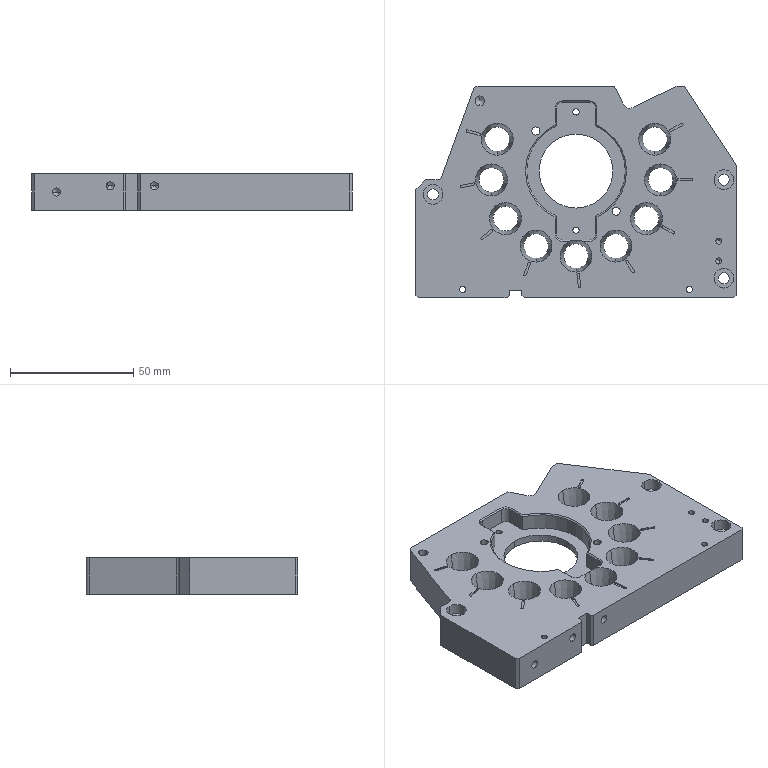NC program | NX | posted with a generic post | part box 130 x 86 x 15 mm
Lines 106 to 1053 of 51277:
(ZLEVEL_PROFILE , TOOL : D10)
N180 T04 M6
N182 G54
N184 G17 G0 G90 X48.294 Y-20.755 B0. C0. S3500 M3
N186 G43 Z30. H4
N188 Z-0.217
N190 G94 G1 X47.012 Y-19.892 F1000.
N192 G3 X46.014 Y-19.823 R1.
N194 G1 X45.265 Y-20.189 F2200.
N196 X39.925 Y-22.793
N198 X39.818 Y-22.842
N200 X47.584 Y-38.764
N202 G2 X48.1 Y-41. R5.1
N204 G1 Y-43.46
N206 G2 X45.347 Y-48.56 R6.1
N208 G1 X14.298 Y-68.936
N210 G2 X10.402 Y-70.1 R7.1
N212 G3 X9.536 Y-70.6 R1.
N214 G1 X8.67 Y-72.1
N216 G0 Z-0.435
N218 G1 X9.536 Y-70.6 F1000.
N220 G2 X10.402 Y-70.1 R1.
N222 G3 X14.298 Y-68.936 R7.1 F2200.
N224 G1 X45.347 Y-48.56
N226 G3 X48.1 Y-43.46 R6.1
N228 G1 Y-41.
N230 G3 X47.584 Y-38.764 R5.1
N232 G1 X39.818 Y-22.842
N234 X39.925 Y-22.793
N236 X45.265 Y-20.189
N238 X46.014 Y-19.823
N240 G2 X47.012 Y-19.892 R1.
N242 G1 X48.294 Y-20.755
N244 G0 Z-0.652
N246 G1 X47.012 Y-19.892 F1000.
N248 G3 X46.014 Y-19.823 R1.
N250 G1 X45.265 Y-20.189 F2200.
N252 X39.925 Y-22.793
N254 X39.818 Y-22.842
N256 X47.584 Y-38.764
N258 G2 X48.1 Y-41. R5.1
N260 G1 Y-43.46
N262 G2 X45.347 Y-48.56 R6.1
N264 G1 X14.298 Y-68.936
N266 G2 X10.402 Y-70.1 R7.1
N268 G3 X9.536 Y-70.6 R1.
N270 G1 X8.67 Y-72.1
N272 G0 Z-0.87
N274 G1 X9.536 Y-70.6 F1000.
N276 G2 X10.402 Y-70.1 R1.
N278 G3 X14.298 Y-68.936 R7.1 F2200.
N280 G1 X45.347 Y-48.56
N282 G3 X48.1 Y-43.46 R6.1
N284 G1 Y-41.
N286 G3 X47.584 Y-38.764 R5.1
N288 G1 X39.818 Y-22.842
N290 X39.925 Y-22.793
N292 X45.265 Y-20.189
N294 X46.014 Y-19.823
N296 G2 X47.012 Y-19.892 R1.
N298 G1 X48.294 Y-20.755
N300 G0 Z-1.087
N302 G1 X47.012 Y-19.892 F1000.
N304 G3 X46.014 Y-19.823 R1.
N306 G1 X45.265 Y-20.189 F2200.
N308 X39.925 Y-22.793
N310 X39.818 Y-22.842
N312 X47.584 Y-38.764
N314 G2 X48.1 Y-41. R5.1
N316 G1 Y-43.46
N318 G2 X45.347 Y-48.56 R6.1
N320 G1 X14.298 Y-68.936
N322 G2 X10.402 Y-70.1 R7.1
N324 G3 X9.536 Y-70.6 R1.
N326 G1 X8.67 Y-72.1
N328 G0 Z-1.304
N330 G1 X9.536 Y-70.6 F1000.
N332 G2 X10.402 Y-70.1 R1.
N334 G3 X14.298 Y-68.936 R7.1 F2200.
N336 G1 X45.347 Y-48.56
N338 G3 X48.1 Y-43.46 R6.1
N340 G1 Y-41.
N342 G3 X47.584 Y-38.764 R5.1
N344 G1 X39.818 Y-22.842
N346 X39.925 Y-22.793
N348 X45.265 Y-20.189
N350 X46.014 Y-19.823
N352 G2 X47.012 Y-19.892 R1.
N354 G1 X48.294 Y-20.755
N356 G0 Z-1.522
N358 G1 X47.012 Y-19.892 F1000.
N360 G3 X46.014 Y-19.823 R1.
N362 G1 X45.265 Y-20.189 F2200.
N364 X39.925 Y-22.793
N366 X39.818 Y-22.842
N368 X47.584 Y-38.764
N370 G2 X48.1 Y-41. R5.1
N372 G1 Y-43.46
N374 G2 X45.347 Y-48.56 R6.1
N376 G1 X14.298 Y-68.936
N378 G2 X10.402 Y-70.1 R7.1
N380 G3 X9.536 Y-70.6 R1.
N382 G1 X8.67 Y-72.1
N384 G0 Z-1.739
N386 G1 X9.536 Y-70.6 F1000.
N388 G2 X10.402 Y-70.1 R1.
N390 G3 X14.298 Y-68.936 R7.1 F2200.
N392 G1 X45.347 Y-48.56
N394 G3 X48.1 Y-43.46 R6.1
N396 G1 Y-41.
N398 G3 X47.584 Y-38.764 R5.1
N400 G1 X39.818 Y-22.842
N402 X39.925 Y-22.793
N404 X45.265 Y-20.189
N406 X46.014 Y-19.823
N408 G2 X47.012 Y-19.892 R1.
N410 G1 X48.294 Y-20.756
N412 G0 Z-1.957
N414 G1 X47.012 Y-19.892 F1000.
N416 G3 X46.014 Y-19.823 R1.
N418 G1 X45.265 Y-20.189 F2200.
N420 X39.925 Y-22.793
N422 X39.818 Y-22.842
N424 X47.584 Y-38.764
N426 G2 X48.1 Y-41. R5.1
N428 G1 Y-43.46
N430 G2 X45.347 Y-48.56 R6.1
N432 G1 X14.298 Y-68.936
N434 G2 X10.402 Y-70.1 R7.1
N436 G3 X9.536 Y-70.6 R1.
N438 G1 X8.67 Y-72.1
N440 G0 Z-2.174
N442 G1 X9.536 Y-70.6 F1000.
N444 G2 X10.402 Y-70.1 R1.
N446 G3 X14.298 Y-68.936 R7.1 F2200.
N448 G1 X45.347 Y-48.56
N450 G3 X48.1 Y-43.46 R6.1
N452 G1 Y-41.
N454 G3 X47.584 Y-38.764 R5.1
N456 G1 X39.818 Y-22.842
N458 X39.925 Y-22.793
N460 X45.265 Y-20.189
N462 X46.014 Y-19.823
N464 G2 X47.012 Y-19.892 R1.
N466 G1 X48.294 Y-20.756
N468 G0 Z-2.391
N470 G1 X47.012 Y-19.892 F1000.
N472 G3 X46.014 Y-19.823 R1.
N474 G1 X45.265 Y-20.189 F2200.
N476 X39.925 Y-22.793
N478 X39.818 Y-22.842
N480 X47.584 Y-38.764
N482 G2 X48.1 Y-41. R5.1
N484 G1 Y-43.46
N486 G2 X45.347 Y-48.56 R6.1
N488 G1 X14.298 Y-68.936
N490 G2 X10.402 Y-70.1 R7.1
N492 G3 X9.536 Y-70.6 R1.
N494 G1 X8.67 Y-72.1
N496 G0 Z-2.609
N498 G1 X9.536 Y-70.6 F1000.
N500 G2 X10.402 Y-70.1 R1.
N502 G3 X14.298 Y-68.936 R7.1 F2200.
N504 G1 X45.347 Y-48.56
N506 G3 X48.1 Y-43.46 R6.1
N508 G1 Y-41.
N510 G3 X47.584 Y-38.764 R5.1
N512 G1 X39.818 Y-22.842
N514 X39.925 Y-22.793
N516 X45.265 Y-20.189
N518 X46.014 Y-19.823
N520 G2 X47.012 Y-19.892 R1.
N522 G1 X48.294 Y-20.756
N524 G0 Z-2.826
N526 G1 X47.012 Y-19.892 F1000.
N528 G3 X46.014 Y-19.823 R1.
N530 G1 X45.265 Y-20.189 F2200.
N532 X39.925 Y-22.793
N534 X39.818 Y-22.842
N536 X47.584 Y-38.764
N538 G2 X48.1 Y-41. R5.1
N540 G1 Y-43.46
N542 G2 X45.347 Y-48.56 R6.1
N544 G1 X14.298 Y-68.936
N546 G2 X10.402 Y-70.1 R7.1
N548 G3 X9.536 Y-70.6 R1.
N550 G1 X8.67 Y-72.1
N552 G0 Z-3.043
N554 G1 X9.536 Y-70.6 F1000.
N556 G2 X10.402 Y-70.1 R1.
N558 G3 X14.298 Y-68.936 R7.1 F2200.
N560 G1 X45.347 Y-48.56
N562 G3 X48.1 Y-43.46 R6.1
N564 G1 Y-41.
N566 G3 X47.584 Y-38.764 R5.1
N568 G1 X39.818 Y-22.842
N570 X39.925 Y-22.793
N572 X45.265 Y-20.189
N574 X46.014 Y-19.823
N576 G2 X47.012 Y-19.892 R1.
N578 G1 X48.294 Y-20.756
N580 G0 Z-3.261
N582 G1 X47.012 Y-19.892 F1000.
N584 G3 X46.014 Y-19.823 R1.
N586 G1 X45.265 Y-20.189 F2200.
N588 X39.925 Y-22.793
N590 X39.818 Y-22.842
N592 X47.584 Y-38.764
N594 G2 X48.1 Y-41. R5.1
N596 G1 Y-43.46
N598 G2 X45.347 Y-48.56 R6.1
N600 G1 X14.298 Y-68.936
N602 G2 X10.402 Y-70.1 R7.1
N604 G3 X9.536 Y-70.6 R1.
N606 G1 X8.67 Y-72.1
N608 G0 Z-3.478
N610 G1 X9.536 Y-70.6 F1000.
N612 G2 X10.402 Y-70.1 R1.
N614 G3 X14.298 Y-68.936 R7.1 F2200.
N616 G1 X45.347 Y-48.56
N618 G3 X48.1 Y-43.46 R6.1
N620 G1 Y-41.
N622 G3 X47.584 Y-38.764 R5.1
N624 G1 X39.818 Y-22.842
N626 X39.925 Y-22.793
N628 X45.265 Y-20.189
N630 X46.014 Y-19.823
N632 G2 X47.012 Y-19.892 R1.
N634 G1 X48.294 Y-20.756
N636 G0 Z-3.696
N638 G1 X47.012 Y-19.892 F1000.
N640 G3 X46.014 Y-19.823 R1.
N642 G1 X45.265 Y-20.189 F2200.
N644 X39.925 Y-22.793
N646 X39.818 Y-22.842
N648 X47.584 Y-38.764
N650 G2 X48.1 Y-41. R5.1
N652 G1 Y-43.46
N654 G2 X45.347 Y-48.56 R6.1
N656 G1 X14.298 Y-68.936
N658 G2 X10.402 Y-70.1 R7.1
N660 G3 X9.536 Y-70.6 R1.
N662 G1 X8.67 Y-72.1
N664 G0 Z-3.913
N666 G1 X9.536 Y-70.6 F1000.
N668 G2 X10.402 Y-70.1 R1.
N670 G3 X14.298 Y-68.936 R7.1 F2200.
N672 G1 X45.347 Y-48.56
N674 G3 X48.1 Y-43.46 R6.1
N676 G1 Y-41.
N678 G3 X47.584 Y-38.764 R5.1
N680 G1 X39.818 Y-22.842
N682 X39.925 Y-22.793
N684 X45.265 Y-20.189
N686 X46.014 Y-19.823
N688 G2 X47.012 Y-19.892 R1.
N690 G1 X48.294 Y-20.756
N692 G0 Z-4.13
N694 G1 X47.012 Y-19.892 F1000.
N696 G3 X46.014 Y-19.823 R1.
N698 G1 X45.265 Y-20.189 F2200.
N700 X39.925 Y-22.793
N702 X39.818 Y-22.842
N704 X47.584 Y-38.764
N706 G2 X48.1 Y-41. R5.1
N708 G1 Y-43.46
N710 G2 X45.347 Y-48.56 R6.1
N712 G1 X14.298 Y-68.936
N714 G2 X10.402 Y-70.1 R7.1
N716 G3 X9.536 Y-70.6 R1.
N718 G1 X8.67 Y-72.1
N720 G0 Z-4.348
N722 G1 X9.536 Y-70.6 F1000.
N724 G2 X10.402 Y-70.1 R1.
N726 G3 X14.298 Y-68.936 R7.1 F2200.
N728 G1 X45.347 Y-48.56
N730 G3 X48.1 Y-43.46 R6.1
N732 G1 Y-41.
N734 G3 X47.584 Y-38.764 R5.1
N736 G1 X39.818 Y-22.842
N738 X39.925 Y-22.793
N740 X45.265 Y-20.189
N742 X46.014 Y-19.823
N744 G2 X47.012 Y-19.892 R1.
N746 G1 X48.294 Y-20.756
N748 G0 Z-4.565
N750 G1 X47.012 Y-19.892 F1000.
N752 G3 X46.014 Y-19.823 R1.
N754 G1 X45.265 Y-20.189 F2200.
N756 X39.925 Y-22.793
N758 X39.818 Y-22.842
N760 X47.584 Y-38.764
N762 G2 X48.1 Y-41. R5.1
N764 G1 Y-43.46
N766 G2 X45.347 Y-48.56 R6.1
N768 G1 X14.298 Y-68.936
N770 G2 X10.402 Y-70.1 R7.1
N772 G3 X9.536 Y-70.6 R1.
N774 G1 X8.67 Y-72.1
N776 G0 Z-4.783
N778 G1 X9.536 Y-70.6 F1000.
N780 G2 X10.402 Y-70.1 R1.
N782 G3 X14.298 Y-68.936 R7.1 F2200.
N784 G1 X45.347 Y-48.56
N786 G3 X48.1 Y-43.46 R6.1
N788 G1 Y-41.
N790 G3 X47.584 Y-38.764 R5.1
N792 G1 X39.818 Y-22.842
N794 X39.925 Y-22.793
N796 X45.265 Y-20.189
N798 X46.014 Y-19.823
N800 G2 X47.012 Y-19.892 R1.
N802 G1 X48.294 Y-20.756
N804 G0 Z-5.
N806 G1 X47.012 Y-19.892 F1000.
N808 G3 X46.014 Y-19.823 R1.
N810 G1 X45.265 Y-20.189 F2200.
N812 X39.925 Y-22.793
N814 X39.818 Y-22.842
N816 X47.584 Y-38.764
N818 G2 X48.1 Y-41. R5.1
N820 G1 Y-43.46
N822 G2 X45.347 Y-48.56 R6.1
N824 G1 X14.298 Y-68.936
N826 G2 X10.402 Y-70.1 R7.1
N828 G3 X9.536 Y-70.6 R1.
N830 G1 X8.67 Y-72.1
N832 G0 Z-5.217
N834 G1 X9.536 Y-70.6 F1000.
N836 G2 X10.402 Y-70.1 R1.
N838 G3 X14.298 Y-68.936 R7.1 F2200.
N840 G1 X45.347 Y-48.56
N842 G3 X48.1 Y-43.46 R6.1
N844 G1 Y-41.
N846 G3 X47.584 Y-38.764 R5.1
N848 G1 X39.818 Y-22.842
N850 X39.925 Y-22.793
N852 X45.265 Y-20.189
N854 X46.014 Y-19.823
N856 G2 X47.012 Y-19.892 R1.
N858 G1 X48.294 Y-20.756
N860 G0 Z-5.435
N862 G1 X47.012 Y-19.892 F1000.
N864 G3 X46.014 Y-19.823 R1.
N866 G1 X45.265 Y-20.189 F2200.
N868 X39.925 Y-22.793
N870 X39.818 Y-22.842
N872 X47.584 Y-38.764
N874 G2 X48.1 Y-41. R5.1
N876 G1 Y-43.46
N878 G2 X45.347 Y-48.56 R6.1
N880 G1 X14.298 Y-68.936
N882 G2 X10.402 Y-70.1 R7.1
N884 G3 X9.536 Y-70.6 R1.
N886 G1 X8.67 Y-72.1
N888 G0 Z-5.652
N890 G1 X9.536 Y-70.6 F1000.
N892 G2 X10.402 Y-70.1 R1.
N894 G3 X14.298 Y-68.936 R7.1 F2200.
N896 G1 X45.347 Y-48.56
N898 G3 X48.1 Y-43.46 R6.1
N900 G1 Y-41.
N902 G3 X47.584 Y-38.764 R5.1
N904 G1 X39.818 Y-22.842
N906 X39.925 Y-22.793
N908 X45.265 Y-20.189
N910 X46.014 Y-19.823
N912 G2 X47.012 Y-19.892 R1.
N914 G1 X48.294 Y-20.756
N916 G0 Z-5.87
N918 G1 X47.012 Y-19.892 F1000.
N920 G3 X46.014 Y-19.823 R1.
N922 G1 X45.265 Y-20.189 F2200.
N924 X39.925 Y-22.793
N926 X39.818 Y-22.842
N928 X47.584 Y-38.764
N930 G2 X48.1 Y-41. R5.1
N932 G1 Y-43.46
N934 G2 X45.347 Y-48.56 R6.1
N936 G1 X14.298 Y-68.936
N938 G2 X10.402 Y-70.1 R7.1
N940 G3 X9.536 Y-70.6 R1.
N942 G1 X8.67 Y-72.1
N944 G0 Z-6.087
N946 G1 X9.536 Y-70.6 F1000.
N948 G2 X10.402 Y-70.1 R1.
N950 G3 X14.298 Y-68.936 R7.1 F2200.
N952 G1 X45.347 Y-48.56
N954 G3 X48.1 Y-43.46 R6.1
N956 G1 Y-41.
N958 G3 X47.584 Y-38.764 R5.1
N960 G1 X39.818 Y-22.842
N962 X39.925 Y-22.793
N964 X45.265 Y-20.189
N966 X46.014 Y-19.823
N968 G2 X47.012 Y-19.892 R1.
N970 G1 X48.294 Y-20.756
N972 G0 Z-6.304
N974 G1 X47.012 Y-19.893 F1000.
N976 G3 X46.014 Y-19.823 R1.
N978 G1 X45.265 Y-20.189 F2200.
N980 X39.925 Y-22.793
N982 X39.818 Y-22.842
N984 X47.584 Y-38.764
N986 G2 X48.1 Y-41. R5.1
N988 G1 Y-43.46
N990 G2 X45.347 Y-48.56 R6.1
N992 G1 X14.298 Y-68.936
N994 G2 X10.402 Y-70.1 R7.1
N996 G3 X9.536 Y-70.6 R1.
N998 G1 X8.67 Y-72.1
N1000 G0 Z-6.522
N1002 G1 X9.536 Y-70.6 F1000.
N1004 G2 X10.402 Y-70.1 R1.
N1006 G3 X14.298 Y-68.936 R7.1 F2200.
N1008 G1 X45.347 Y-48.56
N1010 G3 X48.1 Y-43.46 R6.1
N1012 G1 Y-41.
N1014 G3 X47.584 Y-38.764 R5.1
N1016 G1 X39.818 Y-22.842
N1018 X39.925 Y-22.793
N1020 X45.265 Y-20.189
N1022 X46.014 Y-19.823
N1024 G2 X47.012 Y-19.893 R1.
N1026 G1 X48.294 Y-20.756
N1028 G0 Z-6.739
N1030 G1 X47.012 Y-19.893 F1000.
N1032 G3 X46.014 Y-19.823 R1.
N1034 G1 X45.265 Y-20.189 F2200.
N1036 X39.925 Y-22.793
N1038 X39.818 Y-22.842
N1040 X47.584 Y-38.764
N1042 G2 X48.1 Y-41. R5.1
N1044 G1 Y-43.46
N1046 G2 X45.347 Y-48.56 R6.1
N1048 G1 X14.298 Y-68.936
N1050 G2 X10.402 Y-70.1 R7.1
N1052 G3 X9.536 Y-70.6 R1.
N1054 G1 X8.67 Y-72.1
N1056 G0 Z-6.957
N1058 G1 X9.536 Y-70.6 F1000.
N1060 G2 X10.402 Y-70.1 R1.
N1062 G3 X14.298 Y-68.936 R7.1 F2200.
N1064 G1 X45.347 Y-48.56
N1066 G3 X48.1 Y-43.46 R6.1
N1068 G1 Y-41.
N1070 G3 X47.584 Y-38.764 R5.1
N1072 G1 X39.818 Y-22.842
N1074 X39.925 Y-22.793
N1076 X45.265 Y-20.189
N1078 X46.014 Y-19.823
N1080 G2 X47.012 Y-19.893 R1.
N1082 G1 X48.294 Y-20.756
N1084 G0 Z-7.174
N1086 G1 X47.012 Y-19.893 F1000.
N1088 G3 X46.014 Y-19.823 R1.
N1090 G1 X45.265 Y-20.189 F2200.
N1092 X39.925 Y-22.793
N1094 X39.818 Y-22.842
N1096 X47.584 Y-38.764
N1098 G2 X48.1 Y-41. R5.1
N1100 G1 Y-43.46
N1102 G2 X45.347 Y-48.56 R6.1
N1104 G1 X14.298 Y-68.936
N1106 G2 X10.402 Y-70.1 R7.1
N1108 G3 X9.536 Y-70.6 R1.
N1110 G1 X8.67 Y-72.1
N1112 G0 Z-7.391
N1114 G1 X9.536 Y-70.6 F1000.
N1116 G2 X10.402 Y-70.1 R1.
N1118 G3 X14.298 Y-68.936 R7.1 F2200.
N1120 G1 X45.347 Y-48.56
N1122 G3 X48.1 Y-43.46 R6.1
N1124 G1 Y-41.
N1126 G3 X47.584 Y-38.764 R5.1
N1128 G1 X39.818 Y-22.842
N1130 X39.925 Y-22.793
N1132 X45.265 Y-20.189
N1134 X46.014 Y-19.823
N1136 G2 X47.012 Y-19.893 R1.
N1138 G1 X48.294 Y-20.756
N1140 G0 Z-7.609
N1142 G1 X47.012 Y-19.893 F1000.
N1144 G3 X46.014 Y-19.823 R1.
N1146 G1 X45.265 Y-20.189 F2200.
N1148 X39.925 Y-22.793
N1150 X39.818 Y-22.842
N1152 X47.584 Y-38.764
N1154 G2 X48.1 Y-41. R5.1
N1156 G1 Y-43.46
N1158 G2 X45.347 Y-48.56 R6.1
N1160 G1 X14.298 Y-68.936
N1162 G2 X10.402 Y-70.1 R7.1
N1164 G3 X9.536 Y-70.6 R1.
N1166 G1 X8.67 Y-72.1
N1168 G0 Z-7.826
N1170 G1 X9.536 Y-70.6 F1000.
N1172 G2 X10.402 Y-70.1 R1.
N1174 G3 X14.298 Y-68.936 R7.1 F2200.
N1176 G1 X45.347 Y-48.56
N1178 G3 X48.1 Y-43.46 R6.1
N1180 G1 Y-41.
N1182 G3 X47.584 Y-38.764 R5.1
N1184 G1 X39.818 Y-22.842
N1186 X39.925 Y-22.793
N1188 X45.265 Y-20.189
N1190 X46.014 Y-19.823
N1192 G2 X47.012 Y-19.893 R1.
N1194 G1 X48.293 Y-20.756
N1196 G0 Z-8.043
N1198 G1 X47.012 Y-19.893 F1000.
N1200 G3 X46.014 Y-19.823 R1.
N1202 G1 X45.265 Y-20.189 F2200.
N1204 X39.925 Y-22.793
N1206 X39.818 Y-22.842
N1208 X47.584 Y-38.764
N1210 G2 X48.1 Y-41. R5.1
N1212 G1 Y-43.46
N1214 G2 X45.347 Y-48.56 R6.1
N1216 G1 X14.298 Y-68.936
N1218 G2 X10.402 Y-70.1 R7.1
N1220 G3 X9.536 Y-70.6 R1.
N1222 G1 X8.67 Y-72.1
N1224 G0 Z-8.261
N1226 G1 X9.536 Y-70.6 F1000.
N1228 G2 X10.402 Y-70.1 R1.
N1230 G3 X14.298 Y-68.936 R7.1 F2200.
N1232 G1 X45.347 Y-48.56
N1234 G3 X48.1 Y-43.46 R6.1
N1236 G1 Y-41.
N1238 G3 X47.584 Y-38.764 R5.1
N1240 G1 X39.818 Y-22.842
N1242 X39.925 Y-22.793
N1244 X45.265 Y-20.189
N1246 X46.014 Y-19.823
N1248 G2 X47.012 Y-19.893 R1.
N1250 G1 X48.293 Y-20.756
N1252 G0 Z-8.478
N1254 G1 X47.012 Y-19.893 F1000.
N1256 G3 X46.014 Y-19.823 R1.
N1258 G1 X45.265 Y-20.189 F2200.
N1260 X39.925 Y-22.793
N1262 X39.818 Y-22.842
N1264 X47.584 Y-38.764
N1266 G2 X48.1 Y-41. R5.1
N1268 G1 Y-43.46
N1270 G2 X45.347 Y-48.56 R6.1
N1272 G1 X14.298 Y-68.936
N1274 G2 X10.402 Y-70.1 R7.1
N1276 G3 X9.536 Y-70.6 R1.
N1278 G1 X8.67 Y-72.1
N1280 G0 Z-8.696
N1282 G1 X9.536 Y-70.6 F1000.
N1284 G2 X10.402 Y-70.1 R1.
N1286 G3 X14.298 Y-68.936 R7.1 F2200.
N1288 G1 X45.347 Y-48.56
N1290 G3 X48.1 Y-43.46 R6.1
N1292 G1 Y-41.
N1294 G3 X47.584 Y-38.764 R5.1
N1296 G1 X39.818 Y-22.842
N1298 X39.925 Y-22.793
N1300 X45.265 Y-20.189
N1302 X46.014 Y-19.823
N1304 G2 X47.012 Y-19.893 R1.
N1306 G1 X48.293 Y-20.756
N1308 G0 Z-8.913
N1310 G1 X47.012 Y-19.893 F1000.
N1312 G3 X46.014 Y-19.823 R1.
N1314 G1 X45.265 Y-20.189 F2200.
N1316 X39.925 Y-22.793
N1318 X39.818 Y-22.842
N1320 X47.584 Y-38.764
N1322 G2 X48.1 Y-41. R5.1
N1324 G1 Y-43.46
N1326 G2 X45.347 Y-48.56 R6.1
N1328 G1 X14.298 Y-68.936
N1330 G2 X10.402 Y-70.1 R7.1
N1332 G3 X9.536 Y-70.6 R1.
N1334 G1 X8.67 Y-72.1
N1336 G0 Z-9.13
N1338 G1 X9.536 Y-70.6 F1000.
N1340 G2 X10.402 Y-70.1 R1.
N1342 G3 X14.298 Y-68.936 R7.1 F2200.
N1344 G1 X45.347 Y-48.56
N1346 G3 X48.1 Y-43.46 R6.1
N1348 G1 Y-41.
N1350 G3 X47.584 Y-38.764 R5.1
N1352 G1 X39.818 Y-22.842
N1354 X39.925 Y-22.793
N1356 X45.265 Y-20.189
N1358 X46.014 Y-19.823
N1360 G2 X47.012 Y-19.893 R1.
N1362 G1 X48.293 Y-20.756
N1364 G0 Z-9.348
N1366 G1 X47.012 Y-19.893 F1000.
N1368 G3 X46.014 Y-19.823 R1.
N1370 G1 X45.265 Y-20.189 F2200.
N1372 X39.925 Y-22.793
N1374 X39.818 Y-22.842
N1376 X47.584 Y-38.764
N1378 G2 X48.1 Y-41. R5.1
N1380 G1 Y-43.46
N1382 G2 X45.347 Y-48.56 R6.1
N1384 G1 X14.298 Y-68.936
N1386 G2 X10.402 Y-70.1 R7.1
N1388 G3 X9.536 Y-70.6 R1.
N1390 G1 X8.67 Y-72.1
N1392 G0 Z-9.565
N1394 G1 X9.536 Y-70.6 F1000.
N1396 G2 X10.402 Y-70.1 R1.
N1398 G3 X14.298 Y-68.936 R7.1 F2200.
N1400 G1 X45.347 Y-48.56
N1402 G3 X48.1 Y-43.46 R6.1
N1404 G1 Y-41.
N1406 G3 X47.584 Y-38.764 R5.1
N1408 G1 X39.818 Y-22.842
N1410 X39.925 Y-22.793
N1412 X45.265 Y-20.189
N1414 X46.014 Y-19.823
N1416 G2 X47.012 Y-19.893 R1.
N1418 G1 X48.293 Y-20.756
N1420 G0 Z-9.783
N1422 G1 X47.012 Y-19.893 F1000.
N1424 G3 X46.014 Y-19.823 R1.
N1426 G1 X45.265 Y-20.189 F2200.
N1428 X39.925 Y-22.793
N1430 X39.818 Y-22.842
N1432 X47.584 Y-38.764
N1434 G2 X48.1 Y-41. R5.1
N1436 G1 Y-43.46
N1438 G2 X45.347 Y-48.56 R6.1
N1440 G1 X14.298 Y-68.936
N1442 G2 X10.402 Y-70.1 R7.1
N1444 G3 X9.536 Y-70.6 R1.
N1446 G1 X8.67 Y-72.1
N1448 G0 Z-10.
N1450 G1 X9.536 Y-70.6 F1000.
N1452 G2 X10.402 Y-70.1 R1.
N1454 G3 X14.298 Y-68.936 R7.1 F2200.
N1456 G1 X45.347 Y-48.56
N1458 G3 X48.1 Y-43.46 R6.1
N1460 G1 Y-41.
N1462 G3 X47.584 Y-38.764 R5.1
N1464 G1 X39.818 Y-22.842
N1466 X39.925 Y-22.793
N1468 X45.265 Y-20.189
N1470 X46.014 Y-19.823
N1472 G2 X47.012 Y-19.893 R1.
N1474 G1 X48.293 Y-20.757
N1476 G0 Z-10.217
N1478 G1 X47.012 Y-19.893 F1000.
N1480 G3 X46.014 Y-19.823 R1.
N1482 G1 X45.265 Y-20.189 F2200.
N1484 X39.925 Y-22.793
N1486 X39.818 Y-22.842
N1488 X47.584 Y-38.764
N1490 G2 X48.1 Y-41. R5.1
N1492 G1 Y-43.46
N1494 G2 X45.347 Y-48.56 R6.1
N1496 G1 X14.298 Y-68.936
N1498 G2 X10.402 Y-70.1 R7.1
N1500 G3 X9.536 Y-70.6 R1.
N1502 G1 X8.67 Y-72.1
N1504 G0 Z-10.435
N1506 G1 X9.536 Y-70.6 F1000.
N1508 G2 X10.402 Y-70.1 R1.
N1510 G3 X14.298 Y-68.936 R7.1 F2200.
N1512 G1 X45.347 Y-48.56
N1514 G3 X48.1 Y-43.46 R6.1
N1516 G1 Y-41.
N1518 G3 X47.584 Y-38.764 R5.1
N1520 G1 X39.818 Y-22.842
N1522 X39.925 Y-22.793
N1524 X45.265 Y-20.189
N1526 X46.014 Y-19.823
N1528 G2 X47.012 Y-19.893 R1.
N1530 G1 X48.293 Y-20.757
N1532 G0 Z-10.652
N1534 G1 X47.012 Y-19.893 F1000.
N1536 G3 X46.014 Y-19.823 R1.
N1538 G1 X45.265 Y-20.189 F2200.
N1540 X39.925 Y-22.793
N1542 X39.818 Y-22.842
N1544 X47.584 Y-38.764
N1546 G2 X48.1 Y-41. R5.1
N1548 G1 Y-43.46
N1550 G2 X45.347 Y-48.56 R6.1
N1552 G1 X14.298 Y-68.936
N1554 G2 X10.402 Y-70.1 R7.1
N1556 G3 X9.536 Y-70.6 R1.
N1558 G1 X8.67 Y-72.1
N1560 G0 Z-10.87
N1562 G1 X9.536 Y-70.6 F1000.
N1564 G2 X10.402 Y-70.1 R1.
N1566 G3 X14.298 Y-68.936 R7.1 F2200.
N1568 G1 X45.347 Y-48.56
N1570 G3 X48.1 Y-43.46 R6.1
N1572 G1 Y-41.
N1574 G3 X47.584 Y-38.764 R5.1
N1576 G1 X39.818 Y-22.842
N1578 X39.925 Y-22.793
N1580 X45.265 Y-20.189
N1582 X46.014 Y-19.823
N1584 G2 X47.012 Y-19.893 R1.
N1586 G1 X48.293 Y-20.757
N1588 G0 Z-11.087
N1590 G1 X47.012 Y-19.893 F1000.
N1592 G3 X46.014 Y-19.823 R1.
N1594 G1 X45.265 Y-20.189 F2200.
N1596 X39.925 Y-22.793
N1598 X39.818 Y-22.842
N1600 X47.584 Y-38.764
N1602 G2 X48.1 Y-41. R5.1
N1604 G1 Y-43.46
N1606 G2 X45.347 Y-48.56 R6.1
N1608 G1 X14.298 Y-68.936
N1610 G2 X10.402 Y-70.1 R7.1
N1612 G3 X9.536 Y-70.6 R1.
N1614 G1 X8.67 Y-72.1
N1616 G0 Z-11.304
N1618 G1 X9.536 Y-70.6 F1000.
N1620 G2 X10.402 Y-70.1 R1.
N1622 G3 X14.298 Y-68.936 R7.1 F2200.
N1624 G1 X45.347 Y-48.56
N1626 G3 X48.1 Y-43.46 R6.1
N1628 G1 Y-41.
N1630 G3 X47.584 Y-38.764 R5.1
N1632 G1 X39.818 Y-22.842
N1634 X39.925 Y-22.793
N1636 X45.265 Y-20.189
N1638 X46.014 Y-19.823
N1640 G2 X47.012 Y-19.893 R1.
N1642 G1 X48.293 Y-20.757
N1644 G0 Z-11.522
N1646 G1 X47.012 Y-19.893 F1000.
N1648 G3 X46.014 Y-19.823 R1.
N1650 G1 X45.265 Y-20.189 F2200.
N1652 X39.925 Y-22.793
N1654 X39.818 Y-22.842
N1656 X47.584 Y-38.764
N1658 G2 X48.1 Y-41. R5.1
N1660 G1 Y-43.46
N1662 G2 X45.347 Y-48.56 R6.1
N1664 G1 X14.298 Y-68.936
N1666 G2 X10.402 Y-70.1 R7.1
N1668 G3 X9.536 Y-70.6 R1.
N1670 G1 X8.67 Y-72.1
N1672 G0 Z-11.739
N1674 G1 X9.536 Y-70.6 F1000.
N1676 G2 X10.402 Y-70.1 R1.
N1678 G3 X14.298 Y-68.936 R7.1 F2200.
N1680 G1 X45.347 Y-48.56
N1682 G3 X48.1 Y-43.46 R6.1
N1684 G1 Y-41.
N1686 G3 X47.584 Y-38.764 R5.1
N1688 G1 X39.818 Y-22.842
N1690 X39.925 Y-22.793
N1692 X45.265 Y-20.189
N1694 X46.014 Y-19.823
N1696 G2 X47.012 Y-19.893 R1.
N1698 G1 X48.293 Y-20.757
N1700 G0 Z-11.957
N1702 G1 X47.012 Y-19.893 F1000.
N1704 G3 X46.014 Y-19.823 R1.
N1706 G1 X45.265 Y-20.189 F2200.
N1708 X39.925 Y-22.793
N1710 X39.818 Y-22.842
N1712 X47.584 Y-38.764
N1714 G2 X48.1 Y-41. R5.1
N1716 G1 Y-43.46
N1718 G2 X45.347 Y-48.56 R6.1
N1720 G1 X14.298 Y-68.936
N1722 G2 X10.402 Y-70.1 R7.1
N1724 G3 X9.536 Y-70.6 R1.
N1726 G1 X8.67 Y-72.1
N1728 G0 Z-12.174
N1730 G1 X9.536 Y-70.6 F1000.
N1732 G2 X10.402 Y-70.1 R1.
N1734 G3 X14.298 Y-68.936 R7.1 F2200.
N1736 G1 X45.347 Y-48.56
N1738 G3 X48.1 Y-43.46 R6.1
N1740 G1 Y-41.
N1742 G3 X47.584 Y-38.764 R5.1
N1744 G1 X39.818 Y-22.842
N1746 X39.925 Y-22.793
N1748 X45.265 Y-20.189
N1750 X46.014 Y-19.823
N1752 G2 X47.012 Y-19.893 R1.
N1754 G1 X48.293 Y-20.757
N1756 G0 Z-12.391
N1758 G1 X47.012 Y-19.893 F1000.
N1760 G3 X46.014 Y-19.823 R1.
N1762 G1 X45.265 Y-20.189 F2200.
N1764 X39.925 Y-22.793
N1766 X39.818 Y-22.842
N1768 X47.584 Y-38.764
N1770 G2 X48.1 Y-41. R5.1
N1772 G1 Y-43.46
N1774 G2 X45.347 Y-48.56 R6.1
N1776 G1 X14.298 Y-68.936
N1778 G2 X10.402 Y-70.1 R7.1
N1780 G3 X9.536 Y-70.6 R1.
N1782 G1 X8.67 Y-72.1
N1784 G0 Z-12.609
N1786 G1 X9.536 Y-70.6 F1000.
N1788 G2 X10.402 Y-70.1 R1.
N1790 G3 X14.298 Y-68.936 R7.1 F2200.
N1792 G1 X45.347 Y-48.56
N1794 G3 X48.1 Y-43.46 R6.1
N1796 G1 Y-41.
N1798 G3 X47.584 Y-38.764 R5.1
N1800 G1 X39.818 Y-22.842
N1802 X39.925 Y-22.793
N1804 X45.265 Y-20.189
N1806 X46.014 Y-19.824
N1808 G2 X47.012 Y-19.893 R1.
N1810 G1 X48.293 Y-20.757
N1812 G0 Z-12.826
N1814 G1 X47.012 Y-19.893 F1000.
N1816 G3 X46.014 Y-19.824 R1.
N1818 G1 X45.265 Y-20.189 F2200.
N1820 X39.925 Y-22.793
N1822 X39.818 Y-22.842
N1824 X47.584 Y-38.764
N1826 G2 X48.1 Y-41. R5.1
N1828 G1 Y-43.46
N1830 G2 X45.347 Y-48.56 R6.1
N1832 G1 X14.298 Y-68.936
N1834 G2 X10.402 Y-70.1 R7.1
N1836 G3 X9.536 Y-70.6 R1.
N1838 G1 X8.67 Y-72.1
N1840 G0 Z-13.043
N1842 G1 X9.536 Y-70.6 F1000.
N1844 G2 X10.402 Y-70.1 R1.
N1846 G3 X14.298 Y-68.936 R7.1 F2200.
N1848 G1 X45.347 Y-48.56
N1850 G3 X48.1 Y-43.46 R6.1
N1852 G1 Y-41.
N1854 G3 X47.584 Y-38.764 R5.1
N1856 G1 X39.818 Y-22.842
N1858 X39.925 Y-22.793
N1860 X45.265 Y-20.189
N1862 X46.014 Y-19.824
N1864 G2 X47.012 Y-19.893 R1.
N1866 G1 X48.293 Y-20.757
N1868 G0 Z-13.261
N1870 G1 X47.012 Y-19.893 F1000.
N1872 G3 X46.014 Y-19.824 R1.
N1874 G1 X45.265 Y-20.189 F2200.
N1876 X39.925 Y-22.793
N1878 X39.818 Y-22.842
N1880 X47.584 Y-38.764
N1882 G2 X48.1 Y-41. R5.1
N1884 G1 Y-43.46
N1886 G2 X45.347 Y-48.56 R6.1
N1888 G1 X14.298 Y-68.936
N1890 G2 X10.402 Y-70.1 R7.1
N1892 G3 X9.536 Y-70.6 R1.
N1894 G1 X8.67 Y-72.1
N1896 G0 Z-13.478
N1898 G1 X9.536 Y-70.6 F1000.
N1900 G2 X10.402 Y-70.1 R1.
N1902 G3 X14.298 Y-68.936 R7.1 F2200.
N1904 G1 X45.347 Y-48.56
N1906 G3 X48.1 Y-43.46 R6.1
N1908 G1 Y-41.
N1910 G3 X47.584 Y-38.764 R5.1
N1912 G1 X39.818 Y-22.842
N1914 X39.925 Y-22.793
N1916 X45.265 Y-20.189
N1918 X46.014 Y-19.824
N1920 G2 X47.012 Y-19.893 R1.
N1922 G1 X48.293 Y-20.757
N1924 G0 Z-13.696
N1926 G1 X47.012 Y-19.893 F1000.
N1928 G3 X46.014 Y-19.824 R1.
N1930 G1 X45.265 Y-20.189 F2200.
N1932 X39.925 Y-22.793
N1934 X39.818 Y-22.842
N1936 X47.584 Y-38.764
N1938 G2 X48.1 Y-41. R5.1
N1940 G1 Y-43.46
N1942 G2 X45.347 Y-48.56 R6.1
N1944 G1 X14.298 Y-68.936
N1946 G2 X10.402 Y-70.1 R7.1
N1948 G3 X9.536 Y-70.6 R1.
N1950 G1 X8.67 Y-72.1
N1952 G0 Z-13.913
N1954 G1 X9.536 Y-70.6 F1000.
N1956 G2 X10.402 Y-70.1 R1.
N1958 G3 X14.298 Y-68.936 R7.1 F2200.
N1960 G1 X45.347 Y-48.56
N1962 G3 X48.1 Y-43.46 R6.1
N1964 G1 Y-41.
N1966 G3 X47.584 Y-38.764 R5.1
N1968 G1 X39.818 Y-22.842
N1970 X39.925 Y-22.793
N1972 X45.265 Y-20.189
N1974 X46.014 Y-19.824
N1976 G2 X47.012 Y-19.893 R1.
N1978 G1 X48.293 Y-20.757
N1980 G0 Z-14.13
N1982 G1 X47.012 Y-19.893 F1000.
N1984 G3 X46.014 Y-19.824 R1.
N1986 G1 X45.265 Y-20.189 F2200.
N1988 X39.925 Y-22.793
N1990 X39.818 Y-22.842
N1992 X47.584 Y-38.764
N1994 G2 X48.1 Y-41. R5.1
N1996 G1 Y-43.46
N1998 G2 X45.347 Y-48.56 R6.1
N2000 G1 X14.298 Y-68.936
N2002 G2 X10.402 Y-70.1 R7.1
N2004 G3 X9.536 Y-70.6 R1.
N2006 G1 X8.67 Y-72.1
N2008 G0 Z-14.348
N2010 G1 X9.536 Y-70.6 F1000.
N2012 G2 X10.402 Y-70.1 R1.
N2014 G3 X14.298 Y-68.936 R7.1 F2200.
N2016 G1 X45.347 Y-48.56
N2018 G3 X48.1 Y-43.46 R6.1
N2020 G1 Y-41.
N2022 G3 X47.584 Y-38.764 R5.1
N2024 G1 X39.818 Y-22.842
N2026 X39.925 Y-22.793
N2028 X45.265 Y-20.189
N2030 X46.014 Y-19.824
N2032 G2 X47.012 Y-19.893 R1.
N2034 G1 X48.293 Y-20.757
N2036 G0 Z-14.565
N2038 G1 X47.012 Y-19.893 F1000.
N2040 G3 X46.014 Y-19.824 R1.
N2042 G1 X45.265 Y-20.189 F2200.
N2044 X39.925 Y-22.793
N2046 X39.818 Y-22.842
N2048 X47.584 Y-38.764
N2050 G2 X48.1 Y-41. R5.1
N2052 G1 Y-43.46
N2054 G2 X45.347 Y-48.56 R6.1
N2056 G1 X14.298 Y-68.936
N2058 G2 X10.402 Y-70.1 R7.1
N2060 G3 X9.536 Y-70.6 R1.
N2062 G1 X8.67 Y-72.1
N2064 G0 Z-14.783
N2066 G1 X9.536 Y-70.6 F1000.
N2068 G2 X10.402 Y-70.1 R1.